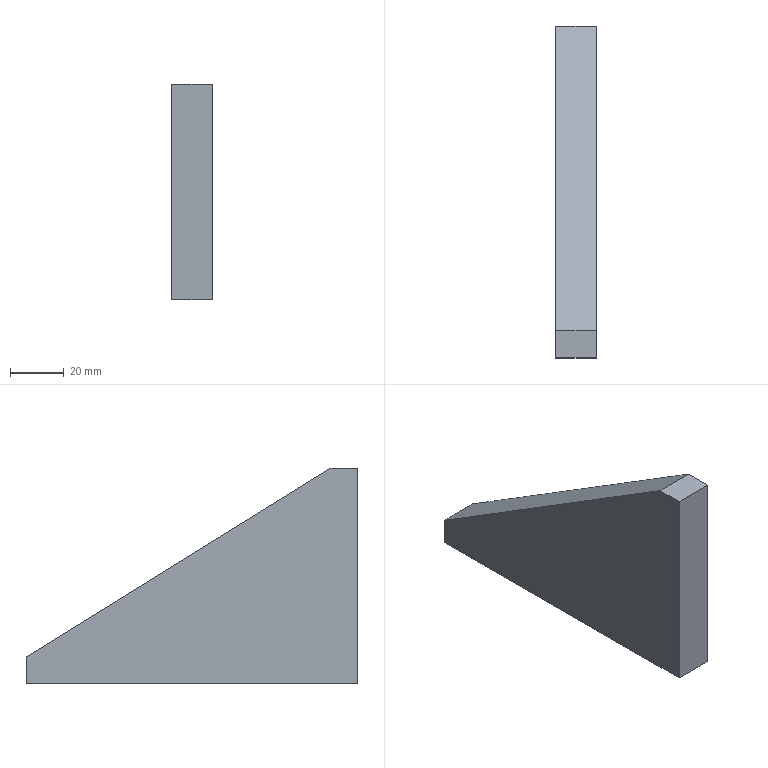Part | NX | features BREP 1, DATUM_CSYS 1 | 1 solid | 7 faces | box 15 x 123 x 80 mm | volume 88275 mm3 | plane 7
STEP:
#1=CARTESIAN_POINT('',(-304.,-57.,224.));
#2=VERTEX_POINT('',#1);
#3=CARTESIAN_POINT('',(-304.,-57.,144.));
#4=VERTEX_POINT('',#3);
#5=CARTESIAN_POINT('',(-304.,-57.,224.));
#6=DIRECTION('',(0.,0.,-1.));
#7=VECTOR('',#6,1000.);
#8=LINE('',#5,#7);
#9=EDGE_CURVE('',#2,#4,#8,.T.);
#10=ORIENTED_EDGE('',*,*,#9,.F.);
#11=CARTESIAN_POINT('',(-319.,-57.,224.));
#12=VERTEX_POINT('',#11);
#13=CARTESIAN_POINT('',(-319.,-57.,224.));
#14=DIRECTION('',(1.,0.,0.));
#15=VECTOR('',#14,1000.);
#16=LINE('',#13,#15);
#17=EDGE_CURVE('',#12,#2,#16,.T.);
#18=ORIENTED_EDGE('',*,*,#17,.F.);
#19=CARTESIAN_POINT('',(-319.,-57.,144.));
#20=VERTEX_POINT('',#19);
#21=CARTESIAN_POINT('',(-319.,-57.,224.));
#22=DIRECTION('',(0.,0.,-1.));
#23=VECTOR('',#22,1000.);
#24=LINE('',#21,#23);
#25=EDGE_CURVE('',#12,#20,#24,.T.);
#26=ORIENTED_EDGE('',*,*,#25,.T.);
#27=CARTESIAN_POINT('',(-319.,-57.,144.));
#28=DIRECTION('',(1.,0.,0.));
#29=VECTOR('',#28,1000.);
#30=LINE('',#27,#29);
#31=EDGE_CURVE('',#20,#4,#30,.T.);
#32=ORIENTED_EDGE('',*,*,#31,.T.);
#33=EDGE_LOOP('',(#10,#18,#26,#32));
#34=FACE_BOUND('',#33,.T.);
#35=CARTESIAN_POINT('',(-319.,-57.,224.));
#36=DIRECTION('',(0.,-1.,0.));
#37=DIRECTION('',(0.,0.,-1.));
#38=AXIS2_PLACEMENT_3D('',#35,#36,#37);
#39=PLANE('',#38);
#40=ADVANCED_FACE('',(#34),#39,.T.);
#41=CARTESIAN_POINT('',(-304.,66.,144.));
#42=VERTEX_POINT('',#41);
#43=CARTESIAN_POINT('',(-304.,-57.,144.));
#44=DIRECTION('',(0.,1.,0.));
#45=VECTOR('',#44,1000.);
#46=LINE('',#43,#45);
#47=EDGE_CURVE('',#4,#42,#46,.T.);
#48=ORIENTED_EDGE('',*,*,#47,.F.);
#49=ORIENTED_EDGE('',*,*,#31,.F.);
#50=CARTESIAN_POINT('',(-319.,66.,144.));
#51=VERTEX_POINT('',#50);
#52=CARTESIAN_POINT('',(-319.,-57.,144.));
#53=DIRECTION('',(0.,1.,0.));
#54=VECTOR('',#53,1000.);
#55=LINE('',#52,#54);
#56=EDGE_CURVE('',#20,#51,#55,.T.);
#57=ORIENTED_EDGE('',*,*,#56,.T.);
#58=CARTESIAN_POINT('',(-319.,66.,144.));
#59=DIRECTION('',(1.,0.,0.));
#60=VECTOR('',#59,1000.);
#61=LINE('',#58,#60);
#62=EDGE_CURVE('',#51,#42,#61,.T.);
#63=ORIENTED_EDGE('',*,*,#62,.T.);
#64=EDGE_LOOP('',(#48,#49,#57,#63));
#65=FACE_BOUND('',#64,.T.);
#66=CARTESIAN_POINT('',(-319.,-57.,144.));
#67=DIRECTION('',(0.,0.,-1.));
#68=DIRECTION('',(-1.,0.,0.));
#69=AXIS2_PLACEMENT_3D('',#66,#67,#68);
#70=PLANE('',#69);
#71=ADVANCED_FACE('',(#65),#70,.T.);
#72=CARTESIAN_POINT('',(-304.,66.,154.));
#73=VERTEX_POINT('',#72);
#74=CARTESIAN_POINT('',(-304.,66.,144.));
#75=DIRECTION('',(0.,0.,1.));
#76=VECTOR('',#75,1000.);
#77=LINE('',#74,#76);
#78=EDGE_CURVE('',#42,#73,#77,.T.);
#79=ORIENTED_EDGE('',*,*,#78,.F.);
#80=ORIENTED_EDGE('',*,*,#62,.F.);
#81=CARTESIAN_POINT('',(-319.,66.,154.));
#82=VERTEX_POINT('',#81);
#83=CARTESIAN_POINT('',(-319.,66.,144.));
#84=DIRECTION('',(0.,0.,1.));
#85=VECTOR('',#84,1000.);
#86=LINE('',#83,#85);
#87=EDGE_CURVE('',#51,#82,#86,.T.);
#88=ORIENTED_EDGE('',*,*,#87,.T.);
#89=CARTESIAN_POINT('',(-319.,66.,154.));
#90=DIRECTION('',(1.,0.,0.));
#91=VECTOR('',#90,1000.);
#92=LINE('',#89,#91);
#93=EDGE_CURVE('',#82,#73,#92,.T.);
#94=ORIENTED_EDGE('',*,*,#93,.T.);
#95=EDGE_LOOP('',(#79,#80,#88,#94));
#96=FACE_BOUND('',#95,.T.);
#97=CARTESIAN_POINT('',(-319.,66.,144.));
#98=DIRECTION('',(0.,1.,0.));
#99=DIRECTION('',(0.,0.,1.));
#100=AXIS2_PLACEMENT_3D('',#97,#98,#99);
#101=PLANE('',#100);
#102=ADVANCED_FACE('',(#96),#101,.T.);
#103=CARTESIAN_POINT('',(-304.,-47.,224.));
#104=VERTEX_POINT('',#103);
#105=CARTESIAN_POINT('',(-304.,66.,154.));
#106=DIRECTION('',(0.,-0.8501,0.5266));
#107=VECTOR('',#106,1000.);
#108=LINE('',#105,#107);
#109=EDGE_CURVE('',#73,#104,#108,.T.);
#110=ORIENTED_EDGE('',*,*,#109,.F.);
#111=ORIENTED_EDGE('',*,*,#93,.F.);
#112=CARTESIAN_POINT('',(-319.,-47.,224.));
#113=VERTEX_POINT('',#112);
#114=CARTESIAN_POINT('',(-319.,66.,154.));
#115=DIRECTION('',(0.,-0.8501,0.5266));
#116=VECTOR('',#115,1000.);
#117=LINE('',#114,#116);
#118=EDGE_CURVE('',#82,#113,#117,.T.);
#119=ORIENTED_EDGE('',*,*,#118,.T.);
#120=CARTESIAN_POINT('',(-319.,-47.,224.));
#121=DIRECTION('',(1.,0.,0.));
#122=VECTOR('',#121,1000.);
#123=LINE('',#120,#122);
#124=EDGE_CURVE('',#113,#104,#123,.T.);
#125=ORIENTED_EDGE('',*,*,#124,.T.);
#126=EDGE_LOOP('',(#110,#111,#119,#125));
#127=FACE_BOUND('',#126,.T.);
#128=CARTESIAN_POINT('',(-319.,66.,154.));
#129=DIRECTION('',(0.,0.5266,0.8501));
#130=DIRECTION('',(0.,-0.8501,0.5266));
#131=AXIS2_PLACEMENT_3D('',#128,#129,#130);
#132=PLANE('',#131);
#133=ADVANCED_FACE('',(#127),#132,.T.);
#134=CARTESIAN_POINT('',(-304.,-47.,224.));
#135=DIRECTION('',(0.,-1.,0.));
#136=VECTOR('',#135,1000.);
#137=LINE('',#134,#136);
#138=EDGE_CURVE('',#104,#2,#137,.T.);
#139=ORIENTED_EDGE('',*,*,#138,.F.);
#140=ORIENTED_EDGE('',*,*,#124,.F.);
#141=CARTESIAN_POINT('',(-319.,-47.,224.));
#142=DIRECTION('',(0.,-1.,0.));
#143=VECTOR('',#142,1000.);
#144=LINE('',#141,#143);
#145=EDGE_CURVE('',#113,#12,#144,.T.);
#146=ORIENTED_EDGE('',*,*,#145,.T.);
#147=ORIENTED_EDGE('',*,*,#17,.T.);
#148=EDGE_LOOP('',(#139,#140,#146,#147));
#149=FACE_BOUND('',#148,.T.);
#150=CARTESIAN_POINT('',(-319.,-47.,224.));
#151=DIRECTION('',(0.,0.,1.));
#152=DIRECTION('',(1.,0.,0.));
#153=AXIS2_PLACEMENT_3D('',#150,#151,#152);
#154=PLANE('',#153);
#155=ADVANCED_FACE('',(#149),#154,.T.);
#156=ORIENTED_EDGE('',*,*,#25,.F.);
#157=ORIENTED_EDGE('',*,*,#145,.F.);
#158=ORIENTED_EDGE('',*,*,#118,.F.);
#159=ORIENTED_EDGE('',*,*,#87,.F.);
#160=ORIENTED_EDGE('',*,*,#56,.F.);
#161=EDGE_LOOP('',(#156,#157,#158,#159,#160));
#162=FACE_BOUND('',#161,.T.);
#163=CARTESIAN_POINT('',(-319.,0.,0.));
#164=DIRECTION('',(1.,0.,0.));
#165=DIRECTION('',(0.,0.,-1.));
#166=AXIS2_PLACEMENT_3D('',#163,#164,#165);
#167=PLANE('',#166);
#168=ADVANCED_FACE('',(#162),#167,.F.);
#169=ORIENTED_EDGE('',*,*,#9,.T.);
#170=ORIENTED_EDGE('',*,*,#47,.T.);
#171=ORIENTED_EDGE('',*,*,#78,.T.);
#172=ORIENTED_EDGE('',*,*,#109,.T.);
#173=ORIENTED_EDGE('',*,*,#138,.T.);
#174=EDGE_LOOP('',(#169,#170,#171,#172,#173));
#175=FACE_BOUND('',#174,.T.);
#176=CARTESIAN_POINT('',(-304.,0.,0.));
#177=DIRECTION('',(1.,0.,0.));
#178=DIRECTION('',(0.,0.,-1.));
#179=AXIS2_PLACEMENT_3D('',#176,#177,#178);
#180=PLANE('',#179);
#181=ADVANCED_FACE('',(#175),#180,.T.);
#182=CLOSED_SHELL('',(#40,#71,#102,#133,#155,#168,#181));
#183=MANIFOLD_SOLID_BREP('',#182);
#184=(LENGTH_UNIT()NAMED_UNIT(*)SI_UNIT(.MILLI.,.METRE.));
#185=UNCERTAINTY_MEASURE_WITH_UNIT(LENGTH_MEASURE(0.00001),#184,'','');
#186=(NAMED_UNIT(*)PLANE_ANGLE_UNIT()SI_UNIT($,.RADIAN.));
#187=(NAMED_UNIT(*)SI_UNIT($,.STERADIAN.)SOLID_ANGLE_UNIT());
#188=(GEOMETRIC_REPRESENTATION_CONTEXT(3)GLOBAL_UNCERTAINTY_ASSIGNED_CONTEXT((#185))GLOBAL_UNIT_ASSIGNED_CONTEXT((#184,#186,#187))REPRESENTATION_CONTEXT('',''));
#189=ADVANCED_BREP_SHAPE_REPRESENTATION('',(#183),#188);